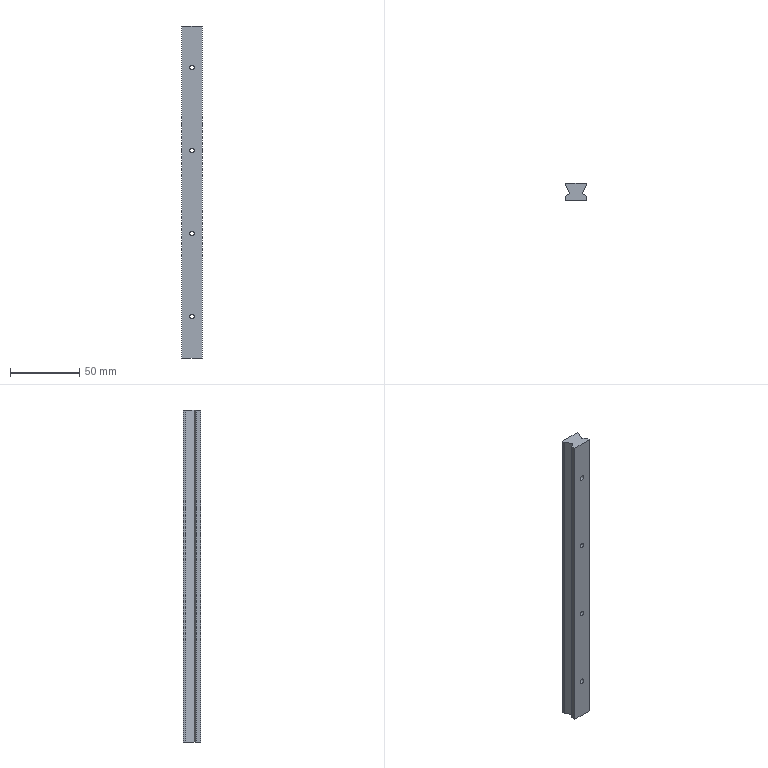Part | STEP file | Mount electronic clip sEGW15SA- slide rail | 1 solid | 32 faces | box 15 x 12.5 x 240 mm | volume 38137 mm3 | cylinder 16 | plane 16 | commonest cylinder face diameters 3.5 x8 7.5 x8